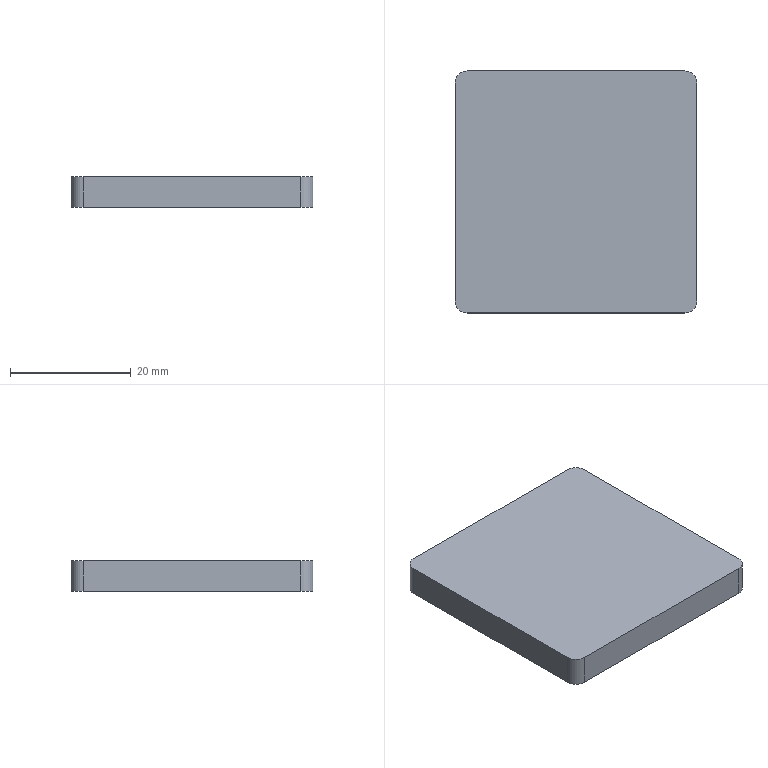Part | SolidWorks | features Extrusion 1 | 1 solid | 10 faces | box 40 x 40 x 5 mm | volume 7983 mm3 | plane 6 | cylinder 4 | commonest cylinder face diameters 4 x4
STEP:
#1=CARTESIAN_POINT('',(0.,2.,0.));
#2=VERTEX_POINT('',#1);
#3=CARTESIAN_POINT('',(2.,0.,0.));
#4=VERTEX_POINT('',#3);
#5=CARTESIAN_POINT('',(2.,2.,0.));
#6=DIRECTION('',(0.,0.,1.));
#7=DIRECTION('',(-1.,0.,0.));
#8=AXIS2_PLACEMENT_3D('',#5,#6,#7);
#9=CIRCLE('',#8,2.);
#10=EDGE_CURVE('',#2,#4,#9,.T.);
#11=ORIENTED_EDGE('',*,*,#10,.T.);
#12=CARTESIAN_POINT('',(2.,0.,5.));
#13=VERTEX_POINT('',#12);
#14=CARTESIAN_POINT('',(2.,0.,5.));
#15=DIRECTION('',(0.,0.,-1.));
#16=VECTOR('',#15,1000.);
#17=LINE('',#14,#16);
#18=EDGE_CURVE('',#13,#4,#17,.T.);
#19=ORIENTED_EDGE('',*,*,#18,.F.);
#20=CARTESIAN_POINT('',(0.,2.,5.));
#21=VERTEX_POINT('',#20);
#22=CARTESIAN_POINT('',(2.,2.,5.));
#23=DIRECTION('',(0.,0.,1.));
#24=DIRECTION('',(-1.,0.,0.));
#25=AXIS2_PLACEMENT_3D('',#22,#23,#24);
#26=CIRCLE('',#25,2.);
#27=EDGE_CURVE('',#21,#13,#26,.T.);
#28=ORIENTED_EDGE('',*,*,#27,.F.);
#29=CARTESIAN_POINT('',(0.,2.,5.));
#30=DIRECTION('',(0.,0.,-1.));
#31=VECTOR('',#30,1000.);
#32=LINE('',#29,#31);
#33=EDGE_CURVE('',#21,#2,#32,.T.);
#34=ORIENTED_EDGE('',*,*,#33,.T.);
#35=EDGE_LOOP('',(#11,#19,#28,#34));
#36=FACE_OUTER_BOUND('',#35,.T.);
#37=CARTESIAN_POINT('',(2.,2.,5.));
#38=DIRECTION('',(0.,0.,-1.));
#39=DIRECTION('',(-1.,0.,0.));
#40=AXIS2_PLACEMENT_3D('',#37,#38,#39);
#41=CYLINDRICAL_SURFACE('',#40,2.);
#42=ADVANCED_FACE('',(#36),#41,.T.);
#43=CARTESIAN_POINT('',(38.,0.,0.));
#44=VERTEX_POINT('',#43);
#45=CARTESIAN_POINT('',(2.,0.,0.));
#46=DIRECTION('',(1.,0.,0.));
#47=VECTOR('',#46,1000.);
#48=LINE('',#45,#47);
#49=EDGE_CURVE('',#4,#44,#48,.T.);
#50=ORIENTED_EDGE('',*,*,#49,.T.);
#51=CARTESIAN_POINT('',(38.,0.,5.));
#52=VERTEX_POINT('',#51);
#53=CARTESIAN_POINT('',(38.,0.,5.));
#54=DIRECTION('',(0.,0.,-1.));
#55=VECTOR('',#54,1000.);
#56=LINE('',#53,#55);
#57=EDGE_CURVE('',#52,#44,#56,.T.);
#58=ORIENTED_EDGE('',*,*,#57,.F.);
#59=CARTESIAN_POINT('',(2.,0.,5.));
#60=DIRECTION('',(1.,0.,0.));
#61=VECTOR('',#60,1000.);
#62=LINE('',#59,#61);
#63=EDGE_CURVE('',#13,#52,#62,.T.);
#64=ORIENTED_EDGE('',*,*,#63,.F.);
#65=ORIENTED_EDGE('',*,*,#18,.T.);
#66=EDGE_LOOP('',(#50,#58,#64,#65));
#67=FACE_OUTER_BOUND('',#66,.T.);
#68=CARTESIAN_POINT('',(2.,0.,5.));
#69=DIRECTION('',(0.,1.,0.));
#70=DIRECTION('',(0.,0.,1.));
#71=AXIS2_PLACEMENT_3D('',#68,#69,#70);
#72=PLANE('',#71);
#73=ADVANCED_FACE('',(#67),#72,.F.);
#74=CARTESIAN_POINT('',(40.,2.,0.));
#75=VERTEX_POINT('',#74);
#76=CARTESIAN_POINT('',(38.,2.,0.));
#77=DIRECTION('',(0.,0.,1.));
#78=DIRECTION('',(-1.,0.,0.));
#79=AXIS2_PLACEMENT_3D('',#76,#77,#78);
#80=CIRCLE('',#79,2.);
#81=EDGE_CURVE('',#44,#75,#80,.T.);
#82=ORIENTED_EDGE('',*,*,#81,.T.);
#83=CARTESIAN_POINT('',(40.,2.,5.));
#84=VERTEX_POINT('',#83);
#85=CARTESIAN_POINT('',(40.,2.,5.));
#86=DIRECTION('',(0.,0.,-1.));
#87=VECTOR('',#86,1000.);
#88=LINE('',#85,#87);
#89=EDGE_CURVE('',#84,#75,#88,.T.);
#90=ORIENTED_EDGE('',*,*,#89,.F.);
#91=CARTESIAN_POINT('',(38.,2.,5.));
#92=DIRECTION('',(0.,0.,1.));
#93=DIRECTION('',(-1.,0.,0.));
#94=AXIS2_PLACEMENT_3D('',#91,#92,#93);
#95=CIRCLE('',#94,2.);
#96=EDGE_CURVE('',#52,#84,#95,.T.);
#97=ORIENTED_EDGE('',*,*,#96,.F.);
#98=ORIENTED_EDGE('',*,*,#57,.T.);
#99=EDGE_LOOP('',(#82,#90,#97,#98));
#100=FACE_OUTER_BOUND('',#99,.T.);
#101=CARTESIAN_POINT('',(38.,2.,5.));
#102=DIRECTION('',(0.,0.,-1.));
#103=DIRECTION('',(-1.,0.,0.));
#104=AXIS2_PLACEMENT_3D('',#101,#102,#103);
#105=CYLINDRICAL_SURFACE('',#104,2.);
#106=ADVANCED_FACE('',(#100),#105,.T.);
#107=CARTESIAN_POINT('',(40.,38.,0.));
#108=VERTEX_POINT('',#107);
#109=CARTESIAN_POINT('',(40.,2.,0.));
#110=DIRECTION('',(0.,1.,0.));
#111=VECTOR('',#110,1000.);
#112=LINE('',#109,#111);
#113=EDGE_CURVE('',#75,#108,#112,.T.);
#114=ORIENTED_EDGE('',*,*,#113,.T.);
#115=CARTESIAN_POINT('',(40.,38.,5.));
#116=VERTEX_POINT('',#115);
#117=CARTESIAN_POINT('',(40.,38.,5.));
#118=DIRECTION('',(0.,0.,-1.));
#119=VECTOR('',#118,1000.);
#120=LINE('',#117,#119);
#121=EDGE_CURVE('',#116,#108,#120,.T.);
#122=ORIENTED_EDGE('',*,*,#121,.F.);
#123=CARTESIAN_POINT('',(40.,2.,5.));
#124=DIRECTION('',(0.,1.,0.));
#125=VECTOR('',#124,1000.);
#126=LINE('',#123,#125);
#127=EDGE_CURVE('',#84,#116,#126,.T.);
#128=ORIENTED_EDGE('',*,*,#127,.F.);
#129=ORIENTED_EDGE('',*,*,#89,.T.);
#130=EDGE_LOOP('',(#114,#122,#128,#129));
#131=FACE_OUTER_BOUND('',#130,.T.);
#132=CARTESIAN_POINT('',(40.,2.,5.));
#133=DIRECTION('',(-1.,0.,0.));
#134=DIRECTION('',(0.,0.,1.));
#135=AXIS2_PLACEMENT_3D('',#132,#133,#134);
#136=PLANE('',#135);
#137=ADVANCED_FACE('',(#131),#136,.F.);
#138=CARTESIAN_POINT('',(38.,40.,0.));
#139=VERTEX_POINT('',#138);
#140=CARTESIAN_POINT('',(38.,38.,0.));
#141=DIRECTION('',(0.,0.,1.));
#142=DIRECTION('',(1.,0.,0.));
#143=AXIS2_PLACEMENT_3D('',#140,#141,#142);
#144=CIRCLE('',#143,2.);
#145=EDGE_CURVE('',#108,#139,#144,.T.);
#146=ORIENTED_EDGE('',*,*,#145,.T.);
#147=CARTESIAN_POINT('',(38.,40.,5.));
#148=VERTEX_POINT('',#147);
#149=CARTESIAN_POINT('',(38.,40.,5.));
#150=DIRECTION('',(0.,0.,-1.));
#151=VECTOR('',#150,1000.);
#152=LINE('',#149,#151);
#153=EDGE_CURVE('',#148,#139,#152,.T.);
#154=ORIENTED_EDGE('',*,*,#153,.F.);
#155=CARTESIAN_POINT('',(38.,38.,5.));
#156=DIRECTION('',(0.,0.,1.));
#157=DIRECTION('',(1.,0.,0.));
#158=AXIS2_PLACEMENT_3D('',#155,#156,#157);
#159=CIRCLE('',#158,2.);
#160=EDGE_CURVE('',#116,#148,#159,.T.);
#161=ORIENTED_EDGE('',*,*,#160,.F.);
#162=ORIENTED_EDGE('',*,*,#121,.T.);
#163=EDGE_LOOP('',(#146,#154,#161,#162));
#164=FACE_OUTER_BOUND('',#163,.T.);
#165=CARTESIAN_POINT('',(38.,38.,5.));
#166=DIRECTION('',(0.,0.,-1.));
#167=DIRECTION('',(-1.,0.,0.));
#168=AXIS2_PLACEMENT_3D('',#165,#166,#167);
#169=CYLINDRICAL_SURFACE('',#168,2.);
#170=ADVANCED_FACE('',(#164),#169,.T.);
#171=CARTESIAN_POINT('',(2.,40.,0.));
#172=VERTEX_POINT('',#171);
#173=CARTESIAN_POINT('',(2.,40.,0.));
#174=DIRECTION('',(-1.,0.,0.));
#175=VECTOR('',#174,1000.);
#176=LINE('',#173,#175);
#177=EDGE_CURVE('',#139,#172,#176,.T.);
#178=ORIENTED_EDGE('',*,*,#177,.T.);
#179=CARTESIAN_POINT('',(2.,40.,5.));
#180=VERTEX_POINT('',#179);
#181=CARTESIAN_POINT('',(2.,40.,5.));
#182=DIRECTION('',(0.,0.,-1.));
#183=VECTOR('',#182,1000.);
#184=LINE('',#181,#183);
#185=EDGE_CURVE('',#180,#172,#184,.T.);
#186=ORIENTED_EDGE('',*,*,#185,.F.);
#187=CARTESIAN_POINT('',(2.,40.,5.));
#188=DIRECTION('',(-1.,0.,0.));
#189=VECTOR('',#188,1000.);
#190=LINE('',#187,#189);
#191=EDGE_CURVE('',#148,#180,#190,.T.);
#192=ORIENTED_EDGE('',*,*,#191,.F.);
#193=ORIENTED_EDGE('',*,*,#153,.T.);
#194=EDGE_LOOP('',(#178,#186,#192,#193));
#195=FACE_OUTER_BOUND('',#194,.T.);
#196=CARTESIAN_POINT('',(2.,40.,5.));
#197=DIRECTION('',(0.,-1.,0.));
#198=DIRECTION('',(0.,0.,-1.));
#199=AXIS2_PLACEMENT_3D('',#196,#197,#198);
#200=PLANE('',#199);
#201=ADVANCED_FACE('',(#195),#200,.F.);
#202=CARTESIAN_POINT('',(0.,38.,0.));
#203=VERTEX_POINT('',#202);
#204=CARTESIAN_POINT('',(2.,38.,0.));
#205=DIRECTION('',(0.,0.,1.));
#206=DIRECTION('',(-1.,0.,0.));
#207=AXIS2_PLACEMENT_3D('',#204,#205,#206);
#208=CIRCLE('',#207,2.);
#209=EDGE_CURVE('',#172,#203,#208,.T.);
#210=ORIENTED_EDGE('',*,*,#209,.T.);
#211=CARTESIAN_POINT('',(0.,38.,5.));
#212=VERTEX_POINT('',#211);
#213=CARTESIAN_POINT('',(0.,38.,5.));
#214=DIRECTION('',(0.,0.,-1.));
#215=VECTOR('',#214,1000.);
#216=LINE('',#213,#215);
#217=EDGE_CURVE('',#212,#203,#216,.T.);
#218=ORIENTED_EDGE('',*,*,#217,.F.);
#219=CARTESIAN_POINT('',(2.,38.,5.));
#220=DIRECTION('',(0.,0.,1.));
#221=DIRECTION('',(-1.,0.,0.));
#222=AXIS2_PLACEMENT_3D('',#219,#220,#221);
#223=CIRCLE('',#222,2.);
#224=EDGE_CURVE('',#180,#212,#223,.T.);
#225=ORIENTED_EDGE('',*,*,#224,.F.);
#226=ORIENTED_EDGE('',*,*,#185,.T.);
#227=EDGE_LOOP('',(#210,#218,#225,#226));
#228=FACE_OUTER_BOUND('',#227,.T.);
#229=CARTESIAN_POINT('',(2.,38.,5.));
#230=DIRECTION('',(0.,0.,-1.));
#231=DIRECTION('',(-1.,0.,0.));
#232=AXIS2_PLACEMENT_3D('',#229,#230,#231);
#233=CYLINDRICAL_SURFACE('',#232,2.);
#234=ADVANCED_FACE('',(#228),#233,.T.);
#235=CARTESIAN_POINT('',(0.,2.,0.));
#236=DIRECTION('',(0.,-1.,0.));
#237=VECTOR('',#236,1000.);
#238=LINE('',#235,#237);
#239=EDGE_CURVE('',#203,#2,#238,.T.);
#240=ORIENTED_EDGE('',*,*,#239,.T.);
#241=ORIENTED_EDGE('',*,*,#33,.F.);
#242=CARTESIAN_POINT('',(0.,2.,5.));
#243=DIRECTION('',(0.,-1.,0.));
#244=VECTOR('',#243,1000.);
#245=LINE('',#242,#244);
#246=EDGE_CURVE('',#212,#21,#245,.T.);
#247=ORIENTED_EDGE('',*,*,#246,.F.);
#248=ORIENTED_EDGE('',*,*,#217,.T.);
#249=EDGE_LOOP('',(#240,#241,#247,#248));
#250=FACE_OUTER_BOUND('',#249,.T.);
#251=CARTESIAN_POINT('',(0.,2.,5.));
#252=DIRECTION('',(1.,0.,0.));
#253=DIRECTION('',(0.,0.,-1.));
#254=AXIS2_PLACEMENT_3D('',#251,#252,#253);
#255=PLANE('',#254);
#256=ADVANCED_FACE('',(#250),#255,.F.);
#257=ORIENTED_EDGE('',*,*,#27,.T.);
#258=ORIENTED_EDGE('',*,*,#63,.T.);
#259=ORIENTED_EDGE('',*,*,#96,.T.);
#260=ORIENTED_EDGE('',*,*,#127,.T.);
#261=ORIENTED_EDGE('',*,*,#160,.T.);
#262=ORIENTED_EDGE('',*,*,#191,.T.);
#263=ORIENTED_EDGE('',*,*,#224,.T.);
#264=ORIENTED_EDGE('',*,*,#246,.T.);
#265=EDGE_LOOP('',(#257,#258,#259,#260,#261,#262,#263,#264));
#266=FACE_OUTER_BOUND('',#265,.T.);
#267=CARTESIAN_POINT('',(2.,2.,5.));
#268=DIRECTION('',(0.,0.,-1.));
#269=DIRECTION('',(-1.,0.,0.));
#270=AXIS2_PLACEMENT_3D('',#267,#268,#269);
#271=PLANE('',#270);
#272=ADVANCED_FACE('',(#266),#271,.F.);
#273=ORIENTED_EDGE('',*,*,#10,.F.);
#274=ORIENTED_EDGE('',*,*,#239,.F.);
#275=ORIENTED_EDGE('',*,*,#209,.F.);
#276=ORIENTED_EDGE('',*,*,#177,.F.);
#277=ORIENTED_EDGE('',*,*,#145,.F.);
#278=ORIENTED_EDGE('',*,*,#113,.F.);
#279=ORIENTED_EDGE('',*,*,#81,.F.);
#280=ORIENTED_EDGE('',*,*,#49,.F.);
#281=EDGE_LOOP('',(#273,#274,#275,#276,#277,#278,#279,#280));
#282=FACE_OUTER_BOUND('',#281,.T.);
#283=CARTESIAN_POINT('',(2.,2.,0.));
#284=DIRECTION('',(0.,0.,-1.));
#285=DIRECTION('',(-1.,0.,0.));
#286=AXIS2_PLACEMENT_3D('',#283,#284,#285);
#287=PLANE('',#286);
#288=ADVANCED_FACE('',(#282),#287,.T.);
#289=CLOSED_SHELL('',(#42,#73,#106,#137,#170,#201,#234,#256,#272,#288));
#290=MANIFOLD_SOLID_BREP('',#289);
#291=CARTESIAN_POINT('',(0.,0.,0.));
#292=DIRECTION('',(0.,0.,1.));
#293=DIRECTION('',(1.,0.,0.));
#294=AXIS2_PLACEMENT_3D('',#291,#292,#293);
#295=(LENGTH_UNIT()NAMED_UNIT(*)SI_UNIT(.MILLI.,.METRE.));
#296=UNCERTAINTY_MEASURE_WITH_UNIT(LENGTH_MEASURE(0.00001),#295,'','');
#297=(NAMED_UNIT(*)PLANE_ANGLE_UNIT()SI_UNIT($,.RADIAN.));
#298=(NAMED_UNIT(*)SI_UNIT($,.STERADIAN.)SOLID_ANGLE_UNIT());
#299=(GEOMETRIC_REPRESENTATION_CONTEXT(3)GLOBAL_UNCERTAINTY_ASSIGNED_CONTEXT((#296))GLOBAL_UNIT_ASSIGNED_CONTEXT((#295,#297,#298))REPRESENTATION_CONTEXT('',''));
#300=ADVANCED_BREP_SHAPE_REPRESENTATION('',(#290,#294),#299);